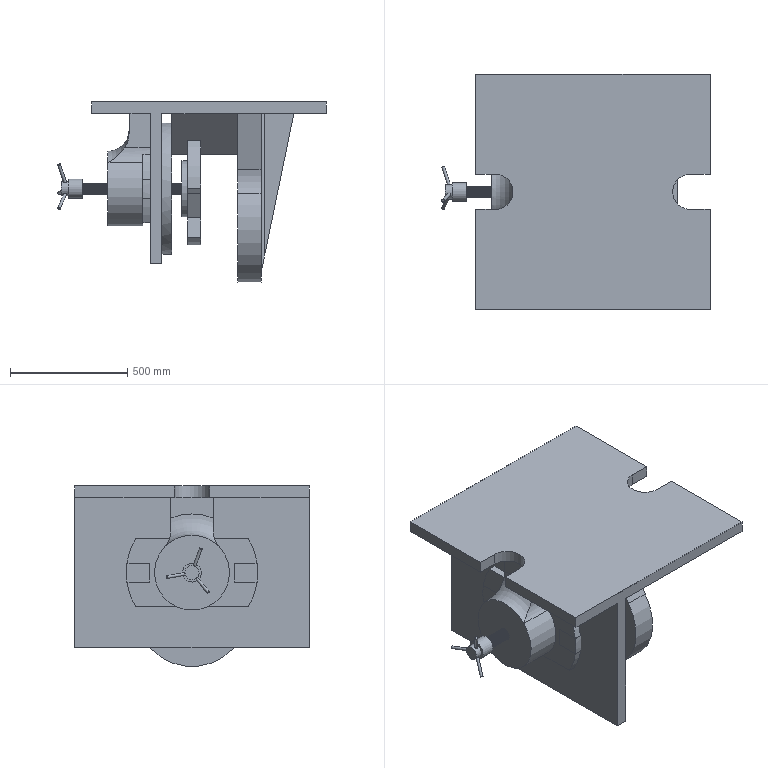Part | NX | features DATUM_CSYS 22, EXTRUDE 14, SKETCH 14, CYLINDER 12, DATUM_PLANE 8, BLEND 5, HELIX 4, SWP104 4, EXTRACT_BODY 2, Pattern Geometry 1, UNITE 1 | 8 solids | 2787 faces | box 1144 x 1000 x 770 mm | volume 170686521 mm3 | torus 2584 | cylinder 120 | plane 83 | commonest cylinder face diameters 48 x90 560 x5 480 x4 12 x3 32 x3 42 x3